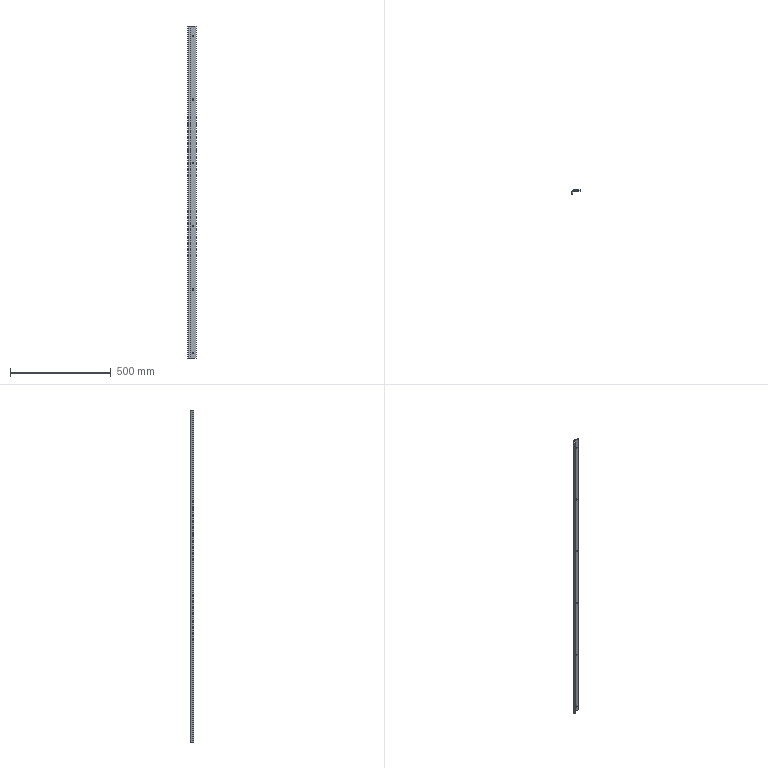Part | SolidWorks | features FlatPattern 1, HoleWzd 1, LPattern 1, SMBaseFlange 1, SheetMetal 1 | 1 solid | 26 faces | box 40 x 19 x 1650 mm | volume 377391 mm3 | cylinder 14 | plane 12 | commonest cylinder face diameters 6.8 x12 12 x1 21 x1
STEP:
#1=CARTESIAN_POINT('',(25.,-4.5,336.6));
#2=VERTEX_POINT('',#1);
#3=CARTESIAN_POINT('',(25.,-4.5,343.4));
#4=VERTEX_POINT('',#3);
#5=CARTESIAN_POINT('',(25.,-4.5,340.));
#6=DIRECTION('',(0.,1.,0.));
#7=DIRECTION('',(0.,0.,1.));
#8=AXIS2_PLACEMENT_3D('',#5,#6,#7);
#9=CIRCLE('',#8,3.4);
#10=EDGE_CURVE('',#2,#4,#9,.T.);
#11=ORIENTED_EDGE('',*,*,#10,.F.);
#12=CARTESIAN_POINT('',(25.,0.,336.6));
#13=VERTEX_POINT('',#12);
#14=CARTESIAN_POINT('',(25.,0.,336.6));
#15=DIRECTION('',(0.,1.,0.));
#16=VECTOR('',#15,1000.);
#17=LINE('',#14,#16);
#18=EDGE_CURVE('',#2,#13,#17,.T.);
#19=ORIENTED_EDGE('',*,*,#18,.T.);
#20=CARTESIAN_POINT('',(25.,0.,343.4));
#21=VERTEX_POINT('',#20);
#22=CARTESIAN_POINT('',(25.,0.,340.));
#23=DIRECTION('',(0.,1.,0.));
#24=DIRECTION('',(0.,0.,1.));
#25=AXIS2_PLACEMENT_3D('',#22,#23,#24);
#26=CIRCLE('',#25,3.4);
#27=EDGE_CURVE('',#13,#21,#26,.T.);
#28=ORIENTED_EDGE('',*,*,#27,.T.);
#29=CARTESIAN_POINT('',(25.,0.,343.4));
#30=DIRECTION('',(0.,1.,0.));
#31=VECTOR('',#30,1000.);
#32=LINE('',#29,#31);
#33=EDGE_CURVE('',#4,#21,#32,.T.);
#34=ORIENTED_EDGE('',*,*,#33,.F.);
#35=EDGE_LOOP('',(#11,#19,#28,#34));
#36=FACE_OUTER_BOUND('',#35,.T.);
#37=CARTESIAN_POINT('',(25.,0.,340.));
#38=DIRECTION('',(0.,1.,0.));
#39=DIRECTION('',(0.,0.,1.));
#40=AXIS2_PLACEMENT_3D('',#37,#38,#39);
#41=CYLINDRICAL_SURFACE('',#40,3.4);
#42=ADVANCED_FACE('',(#36),#41,.F.);
#43=CARTESIAN_POINT('',(25.,-4.5,21.6));
#44=VERTEX_POINT('',#43);
#45=CARTESIAN_POINT('',(25.,-4.5,28.4));
#46=VERTEX_POINT('',#45);
#47=CARTESIAN_POINT('',(25.,-4.5,25.));
#48=DIRECTION('',(0.,1.,0.));
#49=DIRECTION('',(0.,0.,1.));
#50=AXIS2_PLACEMENT_3D('',#47,#48,#49);
#51=CIRCLE('',#50,3.4);
#52=EDGE_CURVE('',#44,#46,#51,.T.);
#53=ORIENTED_EDGE('',*,*,#52,.F.);
#54=CARTESIAN_POINT('',(25.,0.,21.6));
#55=VERTEX_POINT('',#54);
#56=CARTESIAN_POINT('',(25.,0.,21.6));
#57=DIRECTION('',(0.,1.,0.));
#58=VECTOR('',#57,1000.);
#59=LINE('',#56,#58);
#60=EDGE_CURVE('',#44,#55,#59,.T.);
#61=ORIENTED_EDGE('',*,*,#60,.T.);
#62=CARTESIAN_POINT('',(25.,0.,28.4));
#63=VERTEX_POINT('',#62);
#64=CARTESIAN_POINT('',(25.,0.,25.));
#65=DIRECTION('',(0.,1.,0.));
#66=DIRECTION('',(0.,0.,1.));
#67=AXIS2_PLACEMENT_3D('',#64,#65,#66);
#68=CIRCLE('',#67,3.4);
#69=EDGE_CURVE('',#55,#63,#68,.T.);
#70=ORIENTED_EDGE('',*,*,#69,.T.);
#71=CARTESIAN_POINT('',(25.,0.,28.4));
#72=DIRECTION('',(0.,1.,0.));
#73=VECTOR('',#72,1000.);
#74=LINE('',#71,#73);
#75=EDGE_CURVE('',#46,#63,#74,.T.);
#76=ORIENTED_EDGE('',*,*,#75,.F.);
#77=EDGE_LOOP('',(#53,#61,#70,#76));
#78=FACE_OUTER_BOUND('',#77,.T.);
#79=CARTESIAN_POINT('',(25.,0.,25.));
#80=DIRECTION('',(0.,1.,0.));
#81=DIRECTION('',(0.,0.,1.));
#82=AXIS2_PLACEMENT_3D('',#79,#80,#81);
#83=CYLINDRICAL_SURFACE('',#82,3.4);
#84=ADVANCED_FACE('',(#78),#83,.F.);
#85=CARTESIAN_POINT('',(25.,-4.5,651.6));
#86=VERTEX_POINT('',#85);
#87=CARTESIAN_POINT('',(25.,-4.5,658.4));
#88=VERTEX_POINT('',#87);
#89=CARTESIAN_POINT('',(25.,-4.5,655.));
#90=DIRECTION('',(0.,1.,0.));
#91=DIRECTION('',(0.,0.,1.));
#92=AXIS2_PLACEMENT_3D('',#89,#90,#91);
#93=CIRCLE('',#92,3.4);
#94=EDGE_CURVE('',#86,#88,#93,.T.);
#95=ORIENTED_EDGE('',*,*,#94,.F.);
#96=CARTESIAN_POINT('',(25.,0.,651.6));
#97=VERTEX_POINT('',#96);
#98=CARTESIAN_POINT('',(25.,0.,651.6));
#99=DIRECTION('',(0.,1.,0.));
#100=VECTOR('',#99,1000.);
#101=LINE('',#98,#100);
#102=EDGE_CURVE('',#86,#97,#101,.T.);
#103=ORIENTED_EDGE('',*,*,#102,.T.);
#104=CARTESIAN_POINT('',(25.,0.,658.4));
#105=VERTEX_POINT('',#104);
#106=CARTESIAN_POINT('',(25.,0.,655.));
#107=DIRECTION('',(0.,1.,0.));
#108=DIRECTION('',(0.,0.,1.));
#109=AXIS2_PLACEMENT_3D('',#106,#107,#108);
#110=CIRCLE('',#109,3.4);
#111=EDGE_CURVE('',#97,#105,#110,.T.);
#112=ORIENTED_EDGE('',*,*,#111,.T.);
#113=CARTESIAN_POINT('',(25.,0.,658.4));
#114=DIRECTION('',(0.,1.,0.));
#115=VECTOR('',#114,1000.);
#116=LINE('',#113,#115);
#117=EDGE_CURVE('',#88,#105,#116,.T.);
#118=ORIENTED_EDGE('',*,*,#117,.F.);
#119=EDGE_LOOP('',(#95,#103,#112,#118));
#120=FACE_OUTER_BOUND('',#119,.T.);
#121=CARTESIAN_POINT('',(25.,0.,655.));
#122=DIRECTION('',(0.,1.,0.));
#123=DIRECTION('',(0.,0.,1.));
#124=AXIS2_PLACEMENT_3D('',#121,#122,#123);
#125=CYLINDRICAL_SURFACE('',#124,3.4);
#126=ADVANCED_FACE('',(#120),#125,.F.);
#127=CARTESIAN_POINT('',(25.,-4.5,966.6));
#128=VERTEX_POINT('',#127);
#129=CARTESIAN_POINT('',(25.,-4.5,973.4));
#130=VERTEX_POINT('',#129);
#131=CARTESIAN_POINT('',(25.,-4.5,970.));
#132=DIRECTION('',(0.,1.,0.));
#133=DIRECTION('',(0.,0.,1.));
#134=AXIS2_PLACEMENT_3D('',#131,#132,#133);
#135=CIRCLE('',#134,3.4);
#136=EDGE_CURVE('',#128,#130,#135,.T.);
#137=ORIENTED_EDGE('',*,*,#136,.F.);
#138=CARTESIAN_POINT('',(25.,0.,966.6));
#139=VERTEX_POINT('',#138);
#140=CARTESIAN_POINT('',(25.,0.,966.6));
#141=DIRECTION('',(0.,1.,0.));
#142=VECTOR('',#141,1000.);
#143=LINE('',#140,#142);
#144=EDGE_CURVE('',#128,#139,#143,.T.);
#145=ORIENTED_EDGE('',*,*,#144,.T.);
#146=CARTESIAN_POINT('',(25.,0.,973.4));
#147=VERTEX_POINT('',#146);
#148=CARTESIAN_POINT('',(25.,0.,970.));
#149=DIRECTION('',(0.,1.,0.));
#150=DIRECTION('',(0.,0.,1.));
#151=AXIS2_PLACEMENT_3D('',#148,#149,#150);
#152=CIRCLE('',#151,3.4);
#153=EDGE_CURVE('',#139,#147,#152,.T.);
#154=ORIENTED_EDGE('',*,*,#153,.T.);
#155=CARTESIAN_POINT('',(25.,0.,973.4));
#156=DIRECTION('',(0.,1.,0.));
#157=VECTOR('',#156,1000.);
#158=LINE('',#155,#157);
#159=EDGE_CURVE('',#130,#147,#158,.T.);
#160=ORIENTED_EDGE('',*,*,#159,.F.);
#161=EDGE_LOOP('',(#137,#145,#154,#160));
#162=FACE_OUTER_BOUND('',#161,.T.);
#163=CARTESIAN_POINT('',(25.,0.,970.));
#164=DIRECTION('',(0.,1.,0.));
#165=DIRECTION('',(0.,0.,1.));
#166=AXIS2_PLACEMENT_3D('',#163,#164,#165);
#167=CYLINDRICAL_SURFACE('',#166,3.4);
#168=ADVANCED_FACE('',(#162),#167,.F.);
#169=CARTESIAN_POINT('',(25.,-4.5,1281.6));
#170=VERTEX_POINT('',#169);
#171=CARTESIAN_POINT('',(25.,-4.5,1288.4));
#172=VERTEX_POINT('',#171);
#173=CARTESIAN_POINT('',(25.,-4.5,1285.));
#174=DIRECTION('',(0.,1.,0.));
#175=DIRECTION('',(0.,0.,1.));
#176=AXIS2_PLACEMENT_3D('',#173,#174,#175);
#177=CIRCLE('',#176,3.4);
#178=EDGE_CURVE('',#170,#172,#177,.T.);
#179=ORIENTED_EDGE('',*,*,#178,.F.);
#180=CARTESIAN_POINT('',(25.,0.,1281.6));
#181=VERTEX_POINT('',#180);
#182=CARTESIAN_POINT('',(25.,0.,1281.6));
#183=DIRECTION('',(0.,1.,0.));
#184=VECTOR('',#183,1000.);
#185=LINE('',#182,#184);
#186=EDGE_CURVE('',#170,#181,#185,.T.);
#187=ORIENTED_EDGE('',*,*,#186,.T.);
#188=CARTESIAN_POINT('',(25.,0.,1288.4));
#189=VERTEX_POINT('',#188);
#190=CARTESIAN_POINT('',(25.,0.,1285.));
#191=DIRECTION('',(0.,1.,0.));
#192=DIRECTION('',(0.,0.,1.));
#193=AXIS2_PLACEMENT_3D('',#190,#191,#192);
#194=CIRCLE('',#193,3.4);
#195=EDGE_CURVE('',#181,#189,#194,.T.);
#196=ORIENTED_EDGE('',*,*,#195,.T.);
#197=CARTESIAN_POINT('',(25.,0.,1288.4));
#198=DIRECTION('',(0.,1.,0.));
#199=VECTOR('',#198,1000.);
#200=LINE('',#197,#199);
#201=EDGE_CURVE('',#172,#189,#200,.T.);
#202=ORIENTED_EDGE('',*,*,#201,.F.);
#203=EDGE_LOOP('',(#179,#187,#196,#202));
#204=FACE_OUTER_BOUND('',#203,.T.);
#205=CARTESIAN_POINT('',(25.,0.,1285.));
#206=DIRECTION('',(0.,1.,0.));
#207=DIRECTION('',(0.,0.,1.));
#208=AXIS2_PLACEMENT_3D('',#205,#206,#207);
#209=CYLINDRICAL_SURFACE('',#208,3.4);
#210=ADVANCED_FACE('',(#204),#209,.F.);
#211=CARTESIAN_POINT('',(25.,-4.5,1596.6));
#212=VERTEX_POINT('',#211);
#213=CARTESIAN_POINT('',(25.,-4.5,1603.4));
#214=VERTEX_POINT('',#213);
#215=CARTESIAN_POINT('',(25.,-4.5,1600.));
#216=DIRECTION('',(0.,1.,0.));
#217=DIRECTION('',(0.,0.,1.));
#218=AXIS2_PLACEMENT_3D('',#215,#216,#217);
#219=CIRCLE('',#218,3.4);
#220=EDGE_CURVE('',#212,#214,#219,.T.);
#221=ORIENTED_EDGE('',*,*,#220,.F.);
#222=CARTESIAN_POINT('',(25.,0.,1596.6));
#223=VERTEX_POINT('',#222);
#224=CARTESIAN_POINT('',(25.,0.,1596.6));
#225=DIRECTION('',(0.,1.,0.));
#226=VECTOR('',#225,1000.);
#227=LINE('',#224,#226);
#228=EDGE_CURVE('',#212,#223,#227,.T.);
#229=ORIENTED_EDGE('',*,*,#228,.T.);
#230=CARTESIAN_POINT('',(25.,0.,1603.4));
#231=VERTEX_POINT('',#230);
#232=CARTESIAN_POINT('',(25.,0.,1600.));
#233=DIRECTION('',(0.,1.,0.));
#234=DIRECTION('',(0.,0.,1.));
#235=AXIS2_PLACEMENT_3D('',#232,#233,#234);
#236=CIRCLE('',#235,3.4);
#237=EDGE_CURVE('',#223,#231,#236,.T.);
#238=ORIENTED_EDGE('',*,*,#237,.T.);
#239=CARTESIAN_POINT('',(25.,0.,1603.4));
#240=DIRECTION('',(0.,1.,0.));
#241=VECTOR('',#240,1000.);
#242=LINE('',#239,#241);
#243=EDGE_CURVE('',#214,#231,#242,.T.);
#244=ORIENTED_EDGE('',*,*,#243,.F.);
#245=EDGE_LOOP('',(#221,#229,#238,#244));
#246=FACE_OUTER_BOUND('',#245,.T.);
#247=CARTESIAN_POINT('',(25.,0.,1600.));
#248=DIRECTION('',(0.,1.,0.));
#249=DIRECTION('',(0.,0.,1.));
#250=AXIS2_PLACEMENT_3D('',#247,#248,#249);
#251=CYLINDRICAL_SURFACE('',#250,3.4);
#252=ADVANCED_FACE('',(#246),#251,.F.);
#253=ORIENTED_EDGE('',*,*,#228,.F.);
#254=CARTESIAN_POINT('',(25.,-4.5,1600.));
#255=DIRECTION('',(0.,1.,0.));
#256=DIRECTION('',(0.,0.,1.));
#257=AXIS2_PLACEMENT_3D('',#254,#255,#256);
#258=CIRCLE('',#257,3.4);
#259=EDGE_CURVE('',#214,#212,#258,.T.);
#260=ORIENTED_EDGE('',*,*,#259,.F.);
#261=ORIENTED_EDGE('',*,*,#243,.T.);
#262=CARTESIAN_POINT('',(25.,0.,1600.));
#263=DIRECTION('',(0.,1.,0.));
#264=DIRECTION('',(0.,0.,1.));
#265=AXIS2_PLACEMENT_3D('',#262,#263,#264);
#266=CIRCLE('',#265,3.4);
#267=EDGE_CURVE('',#231,#223,#266,.T.);
#268=ORIENTED_EDGE('',*,*,#267,.T.);
#269=EDGE_LOOP('',(#253,#260,#261,#268));
#270=FACE_OUTER_BOUND('',#269,.T.);
#271=CARTESIAN_POINT('',(25.,0.,1600.));
#272=DIRECTION('',(0.,1.,0.));
#273=DIRECTION('',(0.,0.,1.));
#274=AXIS2_PLACEMENT_3D('',#271,#272,#273);
#275=CYLINDRICAL_SURFACE('',#274,3.4);
#276=ADVANCED_FACE('',(#270),#275,.F.);
#277=ORIENTED_EDGE('',*,*,#186,.F.);
#278=CARTESIAN_POINT('',(25.,-4.5,1285.));
#279=DIRECTION('',(0.,1.,0.));
#280=DIRECTION('',(0.,0.,1.));
#281=AXIS2_PLACEMENT_3D('',#278,#279,#280);
#282=CIRCLE('',#281,3.4);
#283=EDGE_CURVE('',#172,#170,#282,.T.);
#284=ORIENTED_EDGE('',*,*,#283,.F.);
#285=ORIENTED_EDGE('',*,*,#201,.T.);
#286=CARTESIAN_POINT('',(25.,0.,1285.));
#287=DIRECTION('',(0.,1.,0.));
#288=DIRECTION('',(0.,0.,1.));
#289=AXIS2_PLACEMENT_3D('',#286,#287,#288);
#290=CIRCLE('',#289,3.4);
#291=EDGE_CURVE('',#189,#181,#290,.T.);
#292=ORIENTED_EDGE('',*,*,#291,.T.);
#293=EDGE_LOOP('',(#277,#284,#285,#292));
#294=FACE_OUTER_BOUND('',#293,.T.);
#295=CARTESIAN_POINT('',(25.,0.,1285.));
#296=DIRECTION('',(0.,1.,0.));
#297=DIRECTION('',(0.,0.,1.));
#298=AXIS2_PLACEMENT_3D('',#295,#296,#297);
#299=CYLINDRICAL_SURFACE('',#298,3.4);
#300=ADVANCED_FACE('',(#294),#299,.F.);
#301=ORIENTED_EDGE('',*,*,#144,.F.);
#302=CARTESIAN_POINT('',(25.,-4.5,970.));
#303=DIRECTION('',(0.,1.,0.));
#304=DIRECTION('',(0.,0.,1.));
#305=AXIS2_PLACEMENT_3D('',#302,#303,#304);
#306=CIRCLE('',#305,3.4);
#307=EDGE_CURVE('',#130,#128,#306,.T.);
#308=ORIENTED_EDGE('',*,*,#307,.F.);
#309=ORIENTED_EDGE('',*,*,#159,.T.);
#310=CARTESIAN_POINT('',(25.,0.,970.));
#311=DIRECTION('',(0.,1.,0.));
#312=DIRECTION('',(0.,0.,1.));
#313=AXIS2_PLACEMENT_3D('',#310,#311,#312);
#314=CIRCLE('',#313,3.4);
#315=EDGE_CURVE('',#147,#139,#314,.T.);
#316=ORIENTED_EDGE('',*,*,#315,.T.);
#317=EDGE_LOOP('',(#301,#308,#309,#316));
#318=FACE_OUTER_BOUND('',#317,.T.);
#319=CARTESIAN_POINT('',(25.,0.,970.));
#320=DIRECTION('',(0.,1.,0.));
#321=DIRECTION('',(0.,0.,1.));
#322=AXIS2_PLACEMENT_3D('',#319,#320,#321);
#323=CYLINDRICAL_SURFACE('',#322,3.4);
#324=ADVANCED_FACE('',(#318),#323,.F.);
#325=ORIENTED_EDGE('',*,*,#102,.F.);
#326=CARTESIAN_POINT('',(25.,-4.5,655.));
#327=DIRECTION('',(0.,1.,0.));
#328=DIRECTION('',(0.,0.,1.));
#329=AXIS2_PLACEMENT_3D('',#326,#327,#328);
#330=CIRCLE('',#329,3.4);
#331=EDGE_CURVE('',#88,#86,#330,.T.);
#332=ORIENTED_EDGE('',*,*,#331,.F.);
#333=ORIENTED_EDGE('',*,*,#117,.T.);
#334=CARTESIAN_POINT('',(25.,0.,655.));
#335=DIRECTION('',(0.,1.,0.));
#336=DIRECTION('',(0.,0.,1.));
#337=AXIS2_PLACEMENT_3D('',#334,#335,#336);
#338=CIRCLE('',#337,3.4);
#339=EDGE_CURVE('',#105,#97,#338,.T.);
#340=ORIENTED_EDGE('',*,*,#339,.T.);
#341=EDGE_LOOP('',(#325,#332,#333,#340));
#342=FACE_OUTER_BOUND('',#341,.T.);
#343=CARTESIAN_POINT('',(25.,0.,655.));
#344=DIRECTION('',(0.,1.,0.));
#345=DIRECTION('',(0.,0.,1.));
#346=AXIS2_PLACEMENT_3D('',#343,#344,#345);
#347=CYLINDRICAL_SURFACE('',#346,3.4);
#348=ADVANCED_FACE('',(#342),#347,.F.);
#349=CARTESIAN_POINT('',(10.5,0.,1650.));
#350=VERTEX_POINT('',#349);
#351=CARTESIAN_POINT('',(10.5,-4.5,1650.));
#352=VERTEX_POINT('',#351);
#353=CARTESIAN_POINT('',(10.5,0.,1650.));
#354=DIRECTION('',(0.,-1.,0.));
#355=VECTOR('',#354,1000.);
#356=LINE('',#353,#355);
#357=EDGE_CURVE('',#350,#352,#356,.T.);
#358=ORIENTED_EDGE('',*,*,#357,.F.);
#359=CARTESIAN_POINT('',(0.,-10.5,1650.));
#360=VERTEX_POINT('',#359);
#361=CARTESIAN_POINT('',(10.5,-10.5,1650.));
#362=DIRECTION('',(0.,0.,-1.));
#363=DIRECTION('',(1.,0.,0.));
#364=AXIS2_PLACEMENT_3D('',#361,#362,#363);
#365=CIRCLE('',#364,10.5);
#366=EDGE_CURVE('',#360,#350,#365,.T.);
#367=ORIENTED_EDGE('',*,*,#366,.F.);
#368=CARTESIAN_POINT('',(4.5,-10.5,1650.));
#369=VERTEX_POINT('',#368);
#370=CARTESIAN_POINT('',(4.5,-10.5,1650.));
#371=DIRECTION('',(-1.,0.,0.));
#372=VECTOR('',#371,1000.);
#373=LINE('',#370,#372);
#374=EDGE_CURVE('',#369,#360,#373,.T.);
#375=ORIENTED_EDGE('',*,*,#374,.F.);
#376=CARTESIAN_POINT('',(10.5,-10.5,1650.));
#377=DIRECTION('',(0.,0.,-1.));
#378=DIRECTION('',(1.,0.,0.));
#379=AXIS2_PLACEMENT_3D('',#376,#377,#378);
#380=CIRCLE('',#379,6.);
#381=EDGE_CURVE('',#369,#352,#380,.T.);
#382=ORIENTED_EDGE('',*,*,#381,.T.);
#383=EDGE_LOOP('',(#358,#367,#375,#382));
#384=FACE_OUTER_BOUND('',#383,.T.);
#385=CARTESIAN_POINT('',(10.5,0.,1650.));
#386=DIRECTION('',(0.,0.,1.));
#387=DIRECTION('',(1.,0.,0.));
#388=AXIS2_PLACEMENT_3D('',#385,#386,#387);
#389=PLANE('',#388);
#390=ADVANCED_FACE('',(#384),#389,.T.);
#391=CARTESIAN_POINT('',(40.,0.,1650.));
#392=VERTEX_POINT('',#391);
#393=CARTESIAN_POINT('',(0.,0.,1650.));
#394=DIRECTION('',(1.,0.,0.));
#395=VECTOR('',#394,1000.);
#396=LINE('',#393,#395);
#397=EDGE_CURVE('',#350,#392,#396,.T.);
#398=ORIENTED_EDGE('',*,*,#397,.F.);
#399=ORIENTED_EDGE('',*,*,#357,.T.);
#400=CARTESIAN_POINT('',(40.,-4.5,1650.));
#401=VERTEX_POINT('',#400);
#402=CARTESIAN_POINT('',(0.,-4.5,1650.));
#403=DIRECTION('',(1.,0.,0.));
#404=VECTOR('',#403,1000.);
#405=LINE('',#402,#404);
#406=EDGE_CURVE('',#352,#401,#405,.T.);
#407=ORIENTED_EDGE('',*,*,#406,.T.);
#408=CARTESIAN_POINT('',(40.,0.,1650.));
#409=DIRECTION('',(0.,-1.,0.));
#410=VECTOR('',#409,1000.);
#411=LINE('',#408,#410);
#412=EDGE_CURVE('',#392,#401,#411,.T.);
#413=ORIENTED_EDGE('',*,*,#412,.F.);
#414=EDGE_LOOP('',(#398,#399,#407,#413));
#415=FACE_OUTER_BOUND('',#414,.T.);
#416=CARTESIAN_POINT('',(4.5,-10.5,1650.));
#417=DIRECTION('',(0.,0.,1.));
#418=DIRECTION('',(1.,0.,0.));
#419=AXIS2_PLACEMENT_3D('',#416,#417,#418);
#420=PLANE('',#419);
#421=ADVANCED_FACE('',(#415),#420,.T.);
#422=CARTESIAN_POINT('',(0.,-10.5,0.));
#423=VERTEX_POINT('',#422);
#424=CARTESIAN_POINT('',(4.5,-10.5,0.));
#425=VERTEX_POINT('',#424);
#426=CARTESIAN_POINT('',(0.,-10.5,0.));
#427=DIRECTION('',(1.,0.,0.));
#428=VECTOR('',#427,1000.);
#429=LINE('',#426,#428);
#430=EDGE_CURVE('',#423,#425,#429,.T.);
#431=ORIENTED_EDGE('',*,*,#430,.F.);
#432=CARTESIAN_POINT('',(10.5,0.,0.));
#433=VERTEX_POINT('',#432);
#434=CARTESIAN_POINT('',(10.5,-10.5,0.));
#435=DIRECTION('',(0.,0.,-1.));
#436=DIRECTION('',(1.,0.,0.));
#437=AXIS2_PLACEMENT_3D('',#434,#435,#436);
#438=CIRCLE('',#437,10.5);
#439=EDGE_CURVE('',#423,#433,#438,.T.);
#440=ORIENTED_EDGE('',*,*,#439,.T.);
#441=CARTESIAN_POINT('',(10.5,-4.5,0.));
#442=VERTEX_POINT('',#441);
#443=CARTESIAN_POINT('',(10.5,-4.5,0.));
#444=DIRECTION('',(0.,1.,0.));
#445=VECTOR('',#444,1000.);
#446=LINE('',#443,#445);
#447=EDGE_CURVE('',#442,#433,#446,.T.);
#448=ORIENTED_EDGE('',*,*,#447,.F.);
#449=CARTESIAN_POINT('',(10.5,-10.5,0.));
#450=DIRECTION('',(0.,0.,-1.));
#451=DIRECTION('',(1.,0.,0.));
#452=AXIS2_PLACEMENT_3D('',#449,#450,#451);
#453=CIRCLE('',#452,6.);
#454=EDGE_CURVE('',#425,#442,#453,.T.);
#455=ORIENTED_EDGE('',*,*,#454,.F.);
#456=EDGE_LOOP('',(#431,#440,#448,#455));
#457=FACE_OUTER_BOUND('',#456,.T.);
#458=CARTESIAN_POINT('',(0.,-10.5,0.));
#459=DIRECTION('',(0.,0.,-1.));
#460=DIRECTION('',(-1.,0.,0.));
#461=AXIS2_PLACEMENT_3D('',#458,#459,#460);
#462=PLANE('',#461);
#463=ADVANCED_FACE('',(#457),#462,.T.);
#464=CARTESIAN_POINT('',(0.,-19.,0.));
#465=VERTEX_POINT('',#464);
#466=CARTESIAN_POINT('',(0.,0.,0.));
#467=DIRECTION('',(0.,1.,0.));
#468=VECTOR('',#467,1000.);
#469=LINE('',#466,#468);
#470=EDGE_CURVE('',#465,#423,#469,.T.);
#471=ORIENTED_EDGE('',*,*,#470,.T.);
#472=ORIENTED_EDGE('',*,*,#430,.T.);
#473=CARTESIAN_POINT('',(4.5,-19.,0.));
#474=VERTEX_POINT('',#473);
#475=CARTESIAN_POINT('',(4.5,0.,0.));
#476=DIRECTION('',(0.,1.,0.));
#477=VECTOR('',#476,1000.);
#478=LINE('',#475,#477);
#479=EDGE_CURVE('',#474,#425,#478,.T.);
#480=ORIENTED_EDGE('',*,*,#479,.F.);
#481=CARTESIAN_POINT('',(4.5,-19.,0.));
#482=DIRECTION('',(-1.,0.,0.));
#483=VECTOR('',#482,1000.);
#484=LINE('',#481,#483);
#485=EDGE_CURVE('',#474,#465,#484,.T.);
#486=ORIENTED_EDGE('',*,*,#485,.T.);
#487=EDGE_LOOP('',(#471,#472,#480,#486));
#488=FACE_OUTER_BOUND('',#487,.T.);
#489=CARTESIAN_POINT('',(10.5,-4.5,0.));
#490=DIRECTION('',(0.,0.,-1.));
#491=DIRECTION('',(-1.,0.,0.));
#492=AXIS2_PLACEMENT_3D('',#489,#490,#491);
#493=PLANE('',#492);
#494=ADVANCED_FACE('',(#488),#493,.T.);
#495=CARTESIAN_POINT('',(25.,-4.5,340.));
#496=DIRECTION('',(0.,1.,0.));
#497=DIRECTION('',(0.,0.,1.));
#498=AXIS2_PLACEMENT_3D('',#495,#496,#497);
#499=CIRCLE('',#498,3.4);
#500=EDGE_CURVE('',#4,#2,#499,.T.);
#501=ORIENTED_EDGE('',*,*,#500,.T.);
#502=ORIENTED_EDGE('',*,*,#10,.T.);
#503=EDGE_LOOP('',(#501,#502));
#504=FACE_BOUND('',#503,.T.);
#505=CARTESIAN_POINT('',(25.,-4.5,25.));
#506=DIRECTION('',(0.,1.,0.));
#507=DIRECTION('',(0.,0.,1.));
#508=AXIS2_PLACEMENT_3D('',#505,#506,#507);
#509=CIRCLE('',#508,3.4);
#510=EDGE_CURVE('',#46,#44,#509,.T.);
#511=ORIENTED_EDGE('',*,*,#510,.T.);
#512=ORIENTED_EDGE('',*,*,#52,.T.);
#513=EDGE_LOOP('',(#511,#512));
#514=FACE_BOUND('',#513,.T.);
#515=CARTESIAN_POINT('',(40.,-4.5,0.));
#516=VERTEX_POINT('',#515);
#517=CARTESIAN_POINT('',(0.,-4.5,0.));
#518=DIRECTION('',(1.,0.,0.));
#519=VECTOR('',#518,1000.);
#520=LINE('',#517,#519);
#521=EDGE_CURVE('',#442,#516,#520,.T.);
#522=ORIENTED_EDGE('',*,*,#521,.T.);
#523=CARTESIAN_POINT('',(40.,-4.5,1650.));
#524=DIRECTION('',(0.,0.,-1.));
#525=VECTOR('',#524,1000.);
#526=LINE('',#523,#525);
#527=EDGE_CURVE('',#401,#516,#526,.T.);
#528=ORIENTED_EDGE('',*,*,#527,.F.);
#529=ORIENTED_EDGE('',*,*,#406,.F.);
#530=CARTESIAN_POINT('',(10.5,-4.5,1650.));
#531=DIRECTION('',(0.,0.,-1.));
#532=VECTOR('',#531,1000.);
#533=LINE('',#530,#532);
#534=EDGE_CURVE('',#352,#442,#533,.T.);
#535=ORIENTED_EDGE('',*,*,#534,.T.);
#536=EDGE_LOOP('',(#522,#528,#529,#535));
#537=FACE_OUTER_BOUND('',#536,.T.);
#538=ORIENTED_EDGE('',*,*,#331,.T.);
#539=ORIENTED_EDGE('',*,*,#94,.T.);
#540=EDGE_LOOP('',(#538,#539));
#541=FACE_BOUND('',#540,.T.);
#542=ORIENTED_EDGE('',*,*,#307,.T.);
#543=ORIENTED_EDGE('',*,*,#136,.T.);
#544=EDGE_LOOP('',(#542,#543));
#545=FACE_BOUND('',#544,.T.);
#546=ORIENTED_EDGE('',*,*,#283,.T.);
#547=ORIENTED_EDGE('',*,*,#178,.T.);
#548=EDGE_LOOP('',(#546,#547));
#549=FACE_BOUND('',#548,.T.);
#550=ORIENTED_EDGE('',*,*,#259,.T.);
#551=ORIENTED_EDGE('',*,*,#220,.T.);
#552=EDGE_LOOP('',(#550,#551));
#553=FACE_BOUND('',#552,.T.);
#554=CARTESIAN_POINT('',(0.,-4.5,1650.));
#555=DIRECTION('',(0.,1.,0.));
#556=DIRECTION('',(0.,0.,1.));
#557=AXIS2_PLACEMENT_3D('',#554,#555,#556);
#558=PLANE('',#557);
#559=ADVANCED_FACE('',(#504,#514,#537,#541,#545,#549,#553),#558,.F.);
#560=CARTESIAN_POINT('',(40.,0.,0.));
#561=VERTEX_POINT('',#560);
#562=CARTESIAN_POINT('',(40.,0.,0.));
#563=DIRECTION('',(0.,-1.,0.));
#564=VECTOR('',#563,1000.);
#565=LINE('',#562,#564);
#566=EDGE_CURVE('',#561,#516,#565,.T.);
#567=ORIENTED_EDGE('',*,*,#566,.F.);
#568=CARTESIAN_POINT('',(40.,0.,1650.));
#569=DIRECTION('',(0.,0.,-1.));
#570=VECTOR('',#569,1000.);
#571=LINE('',#568,#570);
#572=EDGE_CURVE('',#392,#561,#571,.T.);
#573=ORIENTED_EDGE('',*,*,#572,.F.);
#574=ORIENTED_EDGE('',*,*,#412,.T.);
#575=ORIENTED_EDGE('',*,*,#527,.T.);
#576=EDGE_LOOP('',(#567,#573,#574,#575));
#577=FACE_OUTER_BOUND('',#576,.T.);
#578=CARTESIAN_POINT('',(40.,0.,1650.));
#579=DIRECTION('',(1.,0.,0.));
#580=DIRECTION('',(0.,0.,-1.));
#581=AXIS2_PLACEMENT_3D('',#578,#579,#580);
#582=PLANE('',#581);
#583=ADVANCED_FACE('',(#577),#582,.T.);
#584=CARTESIAN_POINT('',(25.,0.,340.));
#585=DIRECTION('',(0.,1.,0.));
#586=DIRECTION('',(0.,0.,1.));
#587=AXIS2_PLACEMENT_3D('',#584,#585,#586);
#588=CIRCLE('',#587,3.4);
#589=EDGE_CURVE('',#21,#13,#588,.T.);
#590=ORIENTED_EDGE('',*,*,#589,.F.);
#591=ORIENTED_EDGE('',*,*,#27,.F.);
#592=EDGE_LOOP('',(#590,#591));
#593=FACE_BOUND('',#592,.T.);
#594=CARTESIAN_POINT('',(25.,0.,25.));
#595=DIRECTION('',(0.,1.,0.));
#596=DIRECTION('',(0.,0.,1.));
#597=AXIS2_PLACEMENT_3D('',#594,#595,#596);
#598=CIRCLE('',#597,3.4);
#599=EDGE_CURVE('',#63,#55,#598,.T.);
#600=ORIENTED_EDGE('',*,*,#599,.F.);
#601=ORIENTED_EDGE('',*,*,#69,.F.);
#602=EDGE_LOOP('',(#600,#601));
#603=FACE_BOUND('',#602,.T.);
#604=CARTESIAN_POINT('',(0.,0.,0.));
#605=DIRECTION('',(1.,0.,0.));
#606=VECTOR('',#605,1000.);
#607=LINE('',#604,#606);
#608=EDGE_CURVE('',#433,#561,#607,.T.);
#609=ORIENTED_EDGE('',*,*,#608,.F.);
#610=CARTESIAN_POINT('',(10.5,0.,1650.));
#611=DIRECTION('',(0.,0.,-1.));
#612=VECTOR('',#611,1000.);
#613=LINE('',#610,#612);
#614=EDGE_CURVE('',#350,#433,#613,.T.);
#615=ORIENTED_EDGE('',*,*,#614,.F.);
#616=ORIENTED_EDGE('',*,*,#397,.T.);
#617=ORIENTED_EDGE('',*,*,#572,.T.);
#618=EDGE_LOOP('',(#609,#615,#616,#617));
#619=FACE_OUTER_BOUND('',#618,.T.);
#620=ORIENTED_EDGE('',*,*,#339,.F.);
#621=ORIENTED_EDGE('',*,*,#111,.F.);
#622=EDGE_LOOP('',(#620,#621));
#623=FACE_BOUND('',#622,.T.);
#624=ORIENTED_EDGE('',*,*,#315,.F.);
#625=ORIENTED_EDGE('',*,*,#153,.F.);
#626=EDGE_LOOP('',(#624,#625));
#627=FACE_BOUND('',#626,.T.);
#628=ORIENTED_EDGE('',*,*,#291,.F.);
#629=ORIENTED_EDGE('',*,*,#195,.F.);
#630=EDGE_LOOP('',(#628,#629));
#631=FACE_BOUND('',#630,.T.);
#632=ORIENTED_EDGE('',*,*,#267,.F.);
#633=ORIENTED_EDGE('',*,*,#237,.F.);
#634=EDGE_LOOP('',(#632,#633));
#635=FACE_BOUND('',#634,.T.);
#636=CARTESIAN_POINT('',(0.,0.,1650.));
#637=DIRECTION('',(0.,1.,0.));
#638=DIRECTION('',(0.,0.,1.));
#639=AXIS2_PLACEMENT_3D('',#636,#637,#638);
#640=PLANE('',#639);
#641=ADVANCED_FACE('',(#593,#603,#619,#623,#627,#631,#635),#640,.T.);
#642=ORIENTED_EDGE('',*,*,#439,.F.);
#643=CARTESIAN_POINT('',(0.,-10.5,1650.));
#644=DIRECTION('',(0.,0.,-1.));
#645=VECTOR('',#644,1000.);
#646=LINE('',#643,#645);
#647=EDGE_CURVE('',#360,#423,#646,.T.);
#648=ORIENTED_EDGE('',*,*,#647,.F.);
#649=ORIENTED_EDGE('',*,*,#366,.T.);
#650=ORIENTED_EDGE('',*,*,#614,.T.);
#651=EDGE_LOOP('',(#642,#648,#649,#650));
#652=FACE_OUTER_BOUND('',#651,.T.);
#653=CARTESIAN_POINT('',(10.5,-10.5,1650.));
#654=DIRECTION('',(0.,0.,-1.));
#655=DIRECTION('',(-1.,0.,0.));
#656=AXIS2_PLACEMENT_3D('',#653,#654,#655);
#657=CYLINDRICAL_SURFACE('',#656,10.5);
#658=ADVANCED_FACE('',(#652),#657,.T.);
#659=ORIENTED_EDGE('',*,*,#470,.F.);
#660=CARTESIAN_POINT('',(0.,-19.,1650.));
#661=VERTEX_POINT('',#660);
#662=CARTESIAN_POINT('',(0.,-19.,1650.));
#663=DIRECTION('',(0.,0.,-1.));
#664=VECTOR('',#663,1000.);
#665=LINE('',#662,#664);
#666=EDGE_CURVE('',#661,#465,#665,.T.);
#667=ORIENTED_EDGE('',*,*,#666,.F.);
#668=CARTESIAN_POINT('',(0.,0.,1650.));
#669=DIRECTION('',(0.,1.,0.));
#670=VECTOR('',#669,1000.);
#671=LINE('',#668,#670);
#672=EDGE_CURVE('',#661,#360,#671,.T.);
#673=ORIENTED_EDGE('',*,*,#672,.T.);
#674=ORIENTED_EDGE('',*,*,#647,.T.);
#675=EDGE_LOOP('',(#659,#667,#673,#674));
#676=FACE_OUTER_BOUND('',#675,.T.);
#677=CARTESIAN_POINT('',(0.,0.,1650.));
#678=DIRECTION('',(-1.,0.,0.));
#679=DIRECTION('',(0.,0.,1.));
#680=AXIS2_PLACEMENT_3D('',#677,#678,#679);
#681=PLANE('',#680);
#682=ADVANCED_FACE('',(#676),#681,.T.);
#683=ORIENTED_EDGE('',*,*,#485,.F.);
#684=CARTESIAN_POINT('',(4.5,-19.,1650.));
#685=VERTEX_POINT('',#684);
#686=CARTESIAN_POINT('',(4.5,-19.,1650.));
#687=DIRECTION('',(0.,0.,-1.));
#688=VECTOR('',#687,1000.);
#689=LINE('',#686,#688);
#690=EDGE_CURVE('',#685,#474,#689,.T.);
#691=ORIENTED_EDGE('',*,*,#690,.F.);
#692=CARTESIAN_POINT('',(4.5,-19.,1650.));
#693=DIRECTION('',(-1.,0.,0.));
#694=VECTOR('',#693,1000.);
#695=LINE('',#692,#694);
#696=EDGE_CURVE('',#685,#661,#695,.T.);
#697=ORIENTED_EDGE('',*,*,#696,.T.);
#698=ORIENTED_EDGE('',*,*,#666,.T.);
#699=EDGE_LOOP('',(#683,#691,#697,#698));
#700=FACE_OUTER_BOUND('',#699,.T.);
#701=CARTESIAN_POINT('',(4.5,-19.,1650.));
#702=DIRECTION('',(0.,-1.,0.));
#703=DIRECTION('',(0.,0.,-1.));
#704=AXIS2_PLACEMENT_3D('',#701,#702,#703);
#705=PLANE('',#704);
#706=ADVANCED_FACE('',(#700),#705,.T.);
#707=ORIENTED_EDGE('',*,*,#479,.T.);
#708=CARTESIAN_POINT('',(4.5,-10.5,1650.));
#709=DIRECTION('',(0.,0.,-1.));
#710=VECTOR('',#709,1000.);
#711=LINE('',#708,#710);
#712=EDGE_CURVE('',#369,#425,#711,.T.);
#713=ORIENTED_EDGE('',*,*,#712,.F.);
#714=CARTESIAN_POINT('',(4.5,0.,1650.));
#715=DIRECTION('',(0.,1.,0.));
#716=VECTOR('',#715,1000.);
#717=LINE('',#714,#716);
#718=EDGE_CURVE('',#685,#369,#717,.T.);
#719=ORIENTED_EDGE('',*,*,#718,.F.);
#720=ORIENTED_EDGE('',*,*,#690,.T.);
#721=EDGE_LOOP('',(#707,#713,#719,#720));
#722=FACE_OUTER_BOUND('',#721,.T.);
#723=CARTESIAN_POINT('',(4.5,0.,1650.));
#724=DIRECTION('',(-1.,0.,0.));
#725=DIRECTION('',(0.,0.,1.));
#726=AXIS2_PLACEMENT_3D('',#723,#724,#725);
#727=PLANE('',#726);
#728=ADVANCED_FACE('',(#722),#727,.F.);
#729=ORIENTED_EDGE('',*,*,#454,.T.);
#730=ORIENTED_EDGE('',*,*,#534,.F.);
#731=ORIENTED_EDGE('',*,*,#381,.F.);
#732=ORIENTED_EDGE('',*,*,#712,.T.);
#733=EDGE_LOOP('',(#729,#730,#731,#732));
#734=FACE_OUTER_BOUND('',#733,.T.);
#735=CARTESIAN_POINT('',(10.5,-10.5,1650.));
#736=DIRECTION('',(0.,0.,-1.));
#737=DIRECTION('',(-1.,0.,0.));
#738=AXIS2_PLACEMENT_3D('',#735,#736,#737);
#739=CYLINDRICAL_SURFACE('',#738,6.);
#740=ADVANCED_FACE('',(#734),#739,.F.);
#741=ORIENTED_EDGE('',*,*,#718,.T.);
#742=ORIENTED_EDGE('',*,*,#374,.T.);
#743=ORIENTED_EDGE('',*,*,#672,.F.);
#744=ORIENTED_EDGE('',*,*,#696,.F.);
#745=EDGE_LOOP('',(#741,#742,#743,#744));
#746=FACE_OUTER_BOUND('',#745,.T.);
#747=CARTESIAN_POINT('',(10.5,-10.5,1650.));
#748=DIRECTION('',(0.,0.,1.));
#749=DIRECTION('',(1.,0.,0.));
#750=AXIS2_PLACEMENT_3D('',#747,#748,#749);
#751=PLANE('',#750);
#752=ADVANCED_FACE('',(#746),#751,.T.);
#753=ORIENTED_EDGE('',*,*,#521,.F.);
#754=ORIENTED_EDGE('',*,*,#447,.T.);
#755=ORIENTED_EDGE('',*,*,#608,.T.);
#756=ORIENTED_EDGE('',*,*,#566,.T.);
#757=EDGE_LOOP('',(#753,#754,#755,#756));
#758=FACE_OUTER_BOUND('',#757,.T.);
#759=CARTESIAN_POINT('',(10.5,-10.5,0.));
#760=DIRECTION('',(0.,0.,1.));
#761=DIRECTION('',(1.,0.,0.));
#762=AXIS2_PLACEMENT_3D('',#759,#760,#761);
#763=PLANE('',#762);
#764=ADVANCED_FACE('',(#758),#763,.F.);
#765=ORIENTED_EDGE('',*,*,#60,.F.);
#766=ORIENTED_EDGE('',*,*,#510,.F.);
#767=ORIENTED_EDGE('',*,*,#75,.T.);
#768=ORIENTED_EDGE('',*,*,#599,.T.);
#769=EDGE_LOOP('',(#765,#766,#767,#768));
#770=FACE_OUTER_BOUND('',#769,.T.);
#771=CARTESIAN_POINT('',(25.,0.,25.));
#772=DIRECTION('',(0.,1.,0.));
#773=DIRECTION('',(0.,0.,1.));
#774=AXIS2_PLACEMENT_3D('',#771,#772,#773);
#775=CYLINDRICAL_SURFACE('',#774,3.4);
#776=ADVANCED_FACE('',(#770),#775,.F.);
#777=ORIENTED_EDGE('',*,*,#18,.F.);
#778=ORIENTED_EDGE('',*,*,#500,.F.);
#779=ORIENTED_EDGE('',*,*,#33,.T.);
#780=ORIENTED_EDGE('',*,*,#589,.T.);
#781=EDGE_LOOP('',(#777,#778,#779,#780));
#782=FACE_OUTER_BOUND('',#781,.T.);
#783=CARTESIAN_POINT('',(25.,0.,340.));
#784=DIRECTION('',(0.,1.,0.));
#785=DIRECTION('',(0.,0.,1.));
#786=AXIS2_PLACEMENT_3D('',#783,#784,#785);
#787=CYLINDRICAL_SURFACE('',#786,3.4);
#788=ADVANCED_FACE('',(#782),#787,.F.);
#789=CLOSED_SHELL('',(#42,#84,#126,#168,#210,#252,#276,#300,#324,#348,#390,#421,#463,#494,#559,#583,#641,#658,#682,#706,#728,#740,#752,#764,#776,#788));
#790=MANIFOLD_SOLID_BREP('',#789);
#791=CARTESIAN_POINT('',(0.,0.,0.));
#792=DIRECTION('',(0.,0.,1.));
#793=DIRECTION('',(1.,0.,0.));
#794=AXIS2_PLACEMENT_3D('',#791,#792,#793);
#795=(LENGTH_UNIT()NAMED_UNIT(*)SI_UNIT(.MILLI.,.METRE.));
#796=UNCERTAINTY_MEASURE_WITH_UNIT(LENGTH_MEASURE(0.00001),#795,'','');
#797=(NAMED_UNIT(*)PLANE_ANGLE_UNIT()SI_UNIT($,.RADIAN.));
#798=(NAMED_UNIT(*)SI_UNIT($,.STERADIAN.)SOLID_ANGLE_UNIT());
#799=(GEOMETRIC_REPRESENTATION_CONTEXT(3)GLOBAL_UNCERTAINTY_ASSIGNED_CONTEXT((#796))GLOBAL_UNIT_ASSIGNED_CONTEXT((#795,#797,#798))REPRESENTATION_CONTEXT('',''));
#800=ADVANCED_BREP_SHAPE_REPRESENTATION('',(#790,#794),#799);